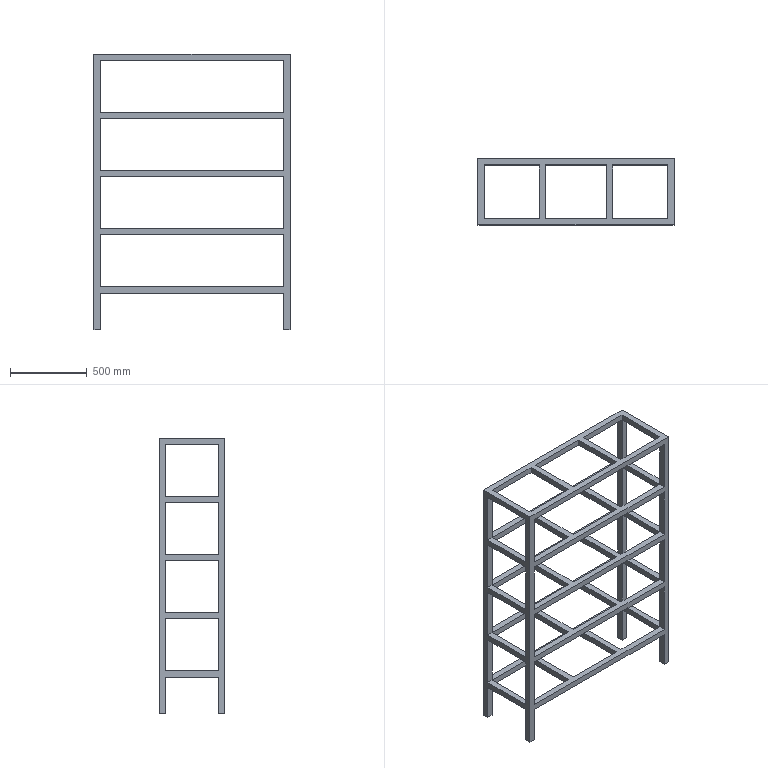Part | SolidWorks | features ICE 4, Extrusion 1 | 1 solid | 136 faces | box 1280 x 430 x 1800 mm | volume 41920000 mm3 | plane 136